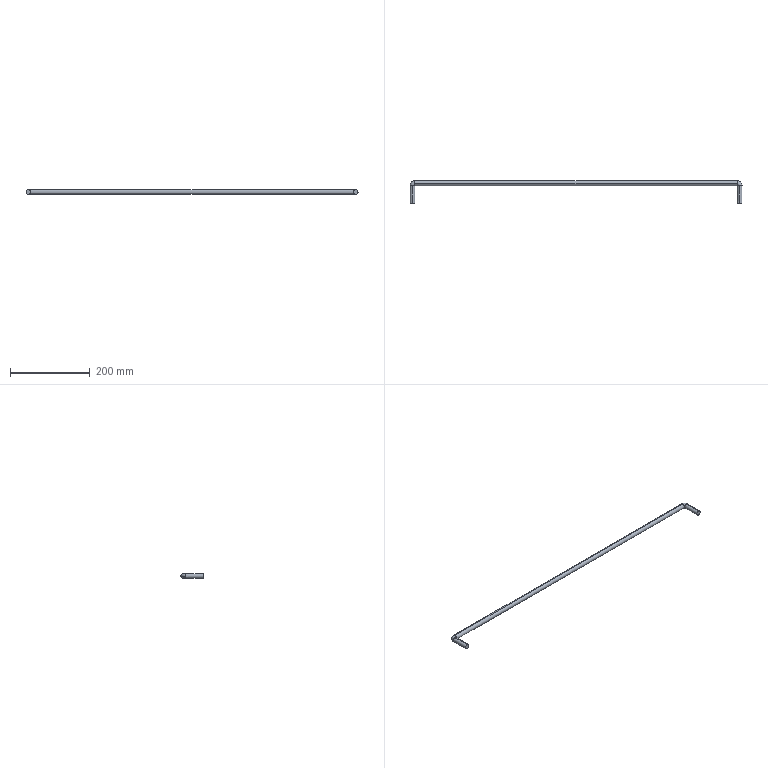Part | SolidWorks | features Sweep 1 | 1 solid | 12 faces | box 831 x 56 x 12 mm | volume 103305 mm3 | cylinder 6 | torus 4 | plane 2 | commonest cylinder face diameters 12 x6
STEP:
#1=CARTESIAN_POINT('',(-49.238,26.641,-6.));
#2=VERTEX_POINT('',#1);
#3=CARTESIAN_POINT('',(-55.238,26.641,0.));
#4=VERTEX_POINT('',#3);
#5=CARTESIAN_POINT('',(-49.238,26.641,0.));
#6=DIRECTION('',(0.,1.,0.));
#7=DIRECTION('',(0.,0.,1.));
#8=AXIS2_PLACEMENT_3D('',#5,#6,#7);
#9=CIRCLE('',#8,6.);
#10=EDGE_CURVE('',#2,#4,#9,.T.);
#11=ORIENTED_EDGE('',*,*,#10,.T.);
#12=CARTESIAN_POINT('',(-42.738,39.141,0.));
#13=VERTEX_POINT('',#12);
#14=CARTESIAN_POINT('',(-42.738,26.641,0.));
#15=DIRECTION('',(0.,0.,-1.));
#16=DIRECTION('',(-1.,0.,0.));
#17=AXIS2_PLACEMENT_3D('',#14,#15,#16);
#18=CIRCLE('',#17,12.5);
#19=EDGE_CURVE('',#4,#13,#18,.T.);
#20=ORIENTED_EDGE('',*,*,#19,.T.);
#21=CARTESIAN_POINT('',(-42.738,33.141,-6.));
#22=VERTEX_POINT('',#21);
#23=CARTESIAN_POINT('',(-42.738,33.141,0.));
#24=DIRECTION('',(1.,0.,0.));
#25=DIRECTION('',(0.,0.,1.));
#26=AXIS2_PLACEMENT_3D('',#23,#24,#25);
#27=CIRCLE('',#26,6.);
#28=EDGE_CURVE('',#22,#13,#27,.T.);
#29=ORIENTED_EDGE('',*,*,#28,.F.);
#30=CARTESIAN_POINT('',(-42.738,27.141,0.));
#31=VERTEX_POINT('',#30);
#32=CARTESIAN_POINT('',(-42.738,33.141,0.));
#33=DIRECTION('',(1.,0.,0.));
#34=DIRECTION('',(0.,0.,1.));
#35=AXIS2_PLACEMENT_3D('',#32,#33,#34);
#36=CIRCLE('',#35,6.);
#37=EDGE_CURVE('',#31,#22,#36,.T.);
#38=ORIENTED_EDGE('',*,*,#37,.F.);
#39=CARTESIAN_POINT('',(-43.238,26.641,0.));
#40=VERTEX_POINT('',#39);
#41=CARTESIAN_POINT('',(-42.738,26.641,0.));
#42=DIRECTION('',(0.,0.,-1.));
#43=DIRECTION('',(-1.,0.,0.));
#44=AXIS2_PLACEMENT_3D('',#41,#42,#43);
#45=CIRCLE('',#44,0.5);
#46=EDGE_CURVE('',#40,#31,#45,.T.);
#47=ORIENTED_EDGE('',*,*,#46,.F.);
#48=CARTESIAN_POINT('',(-49.238,26.641,0.));
#49=DIRECTION('',(0.,1.,0.));
#50=DIRECTION('',(0.,0.,1.));
#51=AXIS2_PLACEMENT_3D('',#48,#49,#50);
#52=CIRCLE('',#51,6.);
#53=EDGE_CURVE('',#40,#2,#52,.T.);
#54=ORIENTED_EDGE('',*,*,#53,.T.);
#55=EDGE_LOOP('',(#11,#20,#29,#38,#47,#54));
#56=FACE_OUTER_BOUND('',#55,.T.);
#57=CARTESIAN_POINT('',(-42.738,26.641,0.));
#58=DIRECTION('',(0.,0.,-1.));
#59=DIRECTION('',(-1.,0.,0.));
#60=AXIS2_PLACEMENT_3D('',#57,#58,#59);
#61=TOROIDAL_SURFACE('',#60,6.5,6.);
#62=ADVANCED_FACE('',(#56),#61,.T.);
#63=CARTESIAN_POINT('',(763.262,33.141,-6.));
#64=VERTEX_POINT('',#63);
#65=CARTESIAN_POINT('',(763.262,39.141,0.));
#66=VERTEX_POINT('',#65);
#67=CARTESIAN_POINT('',(763.262,33.141,0.));
#68=DIRECTION('',(1.,0.,0.));
#69=DIRECTION('',(0.,0.,1.));
#70=AXIS2_PLACEMENT_3D('',#67,#68,#69);
#71=CIRCLE('',#70,6.);
#72=EDGE_CURVE('',#64,#66,#71,.T.);
#73=ORIENTED_EDGE('',*,*,#72,.T.);
#74=CARTESIAN_POINT('',(775.762,26.641,0.));
#75=VERTEX_POINT('',#74);
#76=CARTESIAN_POINT('',(763.262,26.641,0.));
#77=DIRECTION('',(0.,0.,-1.));
#78=DIRECTION('',(-1.,0.,0.));
#79=AXIS2_PLACEMENT_3D('',#76,#77,#78);
#80=CIRCLE('',#79,12.5);
#81=EDGE_CURVE('',#66,#75,#80,.T.);
#82=ORIENTED_EDGE('',*,*,#81,.T.);
#83=CARTESIAN_POINT('',(769.762,26.641,-6.));
#84=VERTEX_POINT('',#83);
#85=CARTESIAN_POINT('',(769.762,26.641,0.));
#86=DIRECTION('',(0.,-1.,0.));
#87=DIRECTION('',(0.,0.,1.));
#88=AXIS2_PLACEMENT_3D('',#85,#86,#87);
#89=CIRCLE('',#88,6.);
#90=EDGE_CURVE('',#84,#75,#89,.T.);
#91=ORIENTED_EDGE('',*,*,#90,.F.);
#92=CARTESIAN_POINT('',(763.762,26.641,0.));
#93=VERTEX_POINT('',#92);
#94=CARTESIAN_POINT('',(769.762,26.641,0.));
#95=DIRECTION('',(0.,-1.,0.));
#96=DIRECTION('',(0.,0.,1.));
#97=AXIS2_PLACEMENT_3D('',#94,#95,#96);
#98=CIRCLE('',#97,6.);
#99=EDGE_CURVE('',#93,#84,#98,.T.);
#100=ORIENTED_EDGE('',*,*,#99,.F.);
#101=CARTESIAN_POINT('',(763.262,27.141,0.));
#102=VERTEX_POINT('',#101);
#103=CARTESIAN_POINT('',(763.262,26.641,0.));
#104=DIRECTION('',(0.,0.,-1.));
#105=DIRECTION('',(-1.,0.,0.));
#106=AXIS2_PLACEMENT_3D('',#103,#104,#105);
#107=CIRCLE('',#106,0.5);
#108=EDGE_CURVE('',#102,#93,#107,.T.);
#109=ORIENTED_EDGE('',*,*,#108,.F.);
#110=CARTESIAN_POINT('',(763.262,33.141,0.));
#111=DIRECTION('',(1.,0.,0.));
#112=DIRECTION('',(0.,0.,1.));
#113=AXIS2_PLACEMENT_3D('',#110,#111,#112);
#114=CIRCLE('',#113,6.);
#115=EDGE_CURVE('',#102,#64,#114,.T.);
#116=ORIENTED_EDGE('',*,*,#115,.T.);
#117=EDGE_LOOP('',(#73,#82,#91,#100,#109,#116));
#118=FACE_OUTER_BOUND('',#117,.T.);
#119=CARTESIAN_POINT('',(763.262,26.641,0.));
#120=DIRECTION('',(0.,0.,-1.));
#121=DIRECTION('',(-1.,0.,0.));
#122=AXIS2_PLACEMENT_3D('',#119,#120,#121);
#123=TOROIDAL_SURFACE('',#122,6.5,6.);
#124=ADVANCED_FACE('',(#118),#123,.T.);
#125=CARTESIAN_POINT('',(-49.238,26.641,6.));
#126=VERTEX_POINT('',#125);
#127=CARTESIAN_POINT('',(-49.238,26.641,0.));
#128=DIRECTION('',(0.,1.,0.));
#129=DIRECTION('',(0.,0.,1.));
#130=AXIS2_PLACEMENT_3D('',#127,#128,#129);
#131=CIRCLE('',#130,6.);
#132=EDGE_CURVE('',#126,#40,#131,.T.);
#133=ORIENTED_EDGE('',*,*,#132,.F.);
#134=CARTESIAN_POINT('',(-49.238,-16.859,6.));
#135=VERTEX_POINT('',#134);
#136=CARTESIAN_POINT('',(-49.238,26.641,6.));
#137=DIRECTION('',(0.,-1.,0.));
#138=VECTOR('',#137,1000.);
#139=LINE('',#136,#138);
#140=EDGE_CURVE('',#126,#135,#139,.T.);
#141=ORIENTED_EDGE('',*,*,#140,.T.);
#142=CARTESIAN_POINT('',(-49.238,-16.859,-6.));
#143=VERTEX_POINT('',#142);
#144=CARTESIAN_POINT('',(-49.238,-16.859,0.));
#145=DIRECTION('',(0.,1.,0.));
#146=DIRECTION('',(0.,0.,1.));
#147=AXIS2_PLACEMENT_3D('',#144,#145,#146);
#148=CIRCLE('',#147,6.);
#149=EDGE_CURVE('',#135,#143,#148,.T.);
#150=ORIENTED_EDGE('',*,*,#149,.T.);
#151=CARTESIAN_POINT('',(-49.238,26.641,-6.));
#152=DIRECTION('',(0.,-1.,0.));
#153=VECTOR('',#152,1000.);
#154=LINE('',#151,#153);
#155=EDGE_CURVE('',#2,#143,#154,.T.);
#156=ORIENTED_EDGE('',*,*,#155,.F.);
#157=ORIENTED_EDGE('',*,*,#53,.F.);
#158=EDGE_LOOP('',(#133,#141,#150,#156,#157));
#159=FACE_OUTER_BOUND('',#158,.T.);
#160=CARTESIAN_POINT('',(-49.238,26.641,0.));
#161=DIRECTION('',(0.,-1.,0.));
#162=DIRECTION('',(0.,0.,-1.));
#163=AXIS2_PLACEMENT_3D('',#160,#161,#162);
#164=CYLINDRICAL_SURFACE('',#163,6.);
#165=ADVANCED_FACE('',(#159),#164,.T.);
#166=ORIENTED_EDGE('',*,*,#28,.T.);
#167=CARTESIAN_POINT('',(-42.738,33.141,6.));
#168=VERTEX_POINT('',#167);
#169=CARTESIAN_POINT('',(-42.738,33.141,0.));
#170=DIRECTION('',(1.,0.,0.));
#171=DIRECTION('',(0.,0.,1.));
#172=AXIS2_PLACEMENT_3D('',#169,#170,#171);
#173=CIRCLE('',#172,6.);
#174=EDGE_CURVE('',#13,#168,#173,.T.);
#175=ORIENTED_EDGE('',*,*,#174,.T.);
#176=CARTESIAN_POINT('',(763.262,33.141,6.));
#177=VERTEX_POINT('',#176);
#178=CARTESIAN_POINT('',(-42.738,33.141,6.));
#179=DIRECTION('',(1.,0.,0.));
#180=VECTOR('',#179,1000.);
#181=LINE('',#178,#180);
#182=EDGE_CURVE('',#168,#177,#181,.T.);
#183=ORIENTED_EDGE('',*,*,#182,.T.);
#184=CARTESIAN_POINT('',(763.262,33.141,0.));
#185=DIRECTION('',(1.,0.,0.));
#186=DIRECTION('',(0.,0.,1.));
#187=AXIS2_PLACEMENT_3D('',#184,#185,#186);
#188=CIRCLE('',#187,6.);
#189=EDGE_CURVE('',#66,#177,#188,.T.);
#190=ORIENTED_EDGE('',*,*,#189,.F.);
#191=ORIENTED_EDGE('',*,*,#72,.F.);
#192=CARTESIAN_POINT('',(-42.738,33.141,-6.));
#193=DIRECTION('',(1.,0.,0.));
#194=VECTOR('',#193,1000.);
#195=LINE('',#192,#194);
#196=EDGE_CURVE('',#22,#64,#195,.T.);
#197=ORIENTED_EDGE('',*,*,#196,.F.);
#198=EDGE_LOOP('',(#166,#175,#183,#190,#191,#197));
#199=FACE_OUTER_BOUND('',#198,.T.);
#200=CARTESIAN_POINT('',(-42.738,33.141,0.));
#201=DIRECTION('',(1.,0.,0.));
#202=DIRECTION('',(0.,0.,-1.));
#203=AXIS2_PLACEMENT_3D('',#200,#201,#202);
#204=CYLINDRICAL_SURFACE('',#203,6.);
#205=ADVANCED_FACE('',(#199),#204,.T.);
#206=ORIENTED_EDGE('',*,*,#90,.T.);
#207=CARTESIAN_POINT('',(769.762,26.641,6.));
#208=VERTEX_POINT('',#207);
#209=CARTESIAN_POINT('',(769.762,26.641,0.));
#210=DIRECTION('',(0.,-1.,0.));
#211=DIRECTION('',(0.,0.,1.));
#212=AXIS2_PLACEMENT_3D('',#209,#210,#211);
#213=CIRCLE('',#212,6.);
#214=EDGE_CURVE('',#75,#208,#213,.T.);
#215=ORIENTED_EDGE('',*,*,#214,.T.);
#216=CARTESIAN_POINT('',(769.762,-16.859,6.));
#217=VERTEX_POINT('',#216);
#218=CARTESIAN_POINT('',(769.762,26.641,6.));
#219=DIRECTION('',(0.,-1.,0.));
#220=VECTOR('',#219,1000.);
#221=LINE('',#218,#220);
#222=EDGE_CURVE('',#208,#217,#221,.T.);
#223=ORIENTED_EDGE('',*,*,#222,.T.);
#224=CARTESIAN_POINT('',(769.762,-16.859,-6.));
#225=VERTEX_POINT('',#224);
#226=CARTESIAN_POINT('',(769.762,-16.859,0.));
#227=DIRECTION('',(0.,-1.,0.));
#228=DIRECTION('',(0.,0.,1.));
#229=AXIS2_PLACEMENT_3D('',#226,#227,#228);
#230=CIRCLE('',#229,6.);
#231=EDGE_CURVE('',#225,#217,#230,.T.);
#232=ORIENTED_EDGE('',*,*,#231,.F.);
#233=CARTESIAN_POINT('',(769.762,26.641,-6.));
#234=DIRECTION('',(0.,-1.,0.));
#235=VECTOR('',#234,1000.);
#236=LINE('',#233,#235);
#237=EDGE_CURVE('',#84,#225,#236,.T.);
#238=ORIENTED_EDGE('',*,*,#237,.F.);
#239=EDGE_LOOP('',(#206,#215,#223,#232,#238));
#240=FACE_OUTER_BOUND('',#239,.T.);
#241=CARTESIAN_POINT('',(769.762,26.641,0.));
#242=DIRECTION('',(0.,-1.,0.));
#243=DIRECTION('',(0.,0.,-1.));
#244=AXIS2_PLACEMENT_3D('',#241,#242,#243);
#245=CYLINDRICAL_SURFACE('',#244,6.);
#246=ADVANCED_FACE('',(#240),#245,.T.);
#247=ORIENTED_EDGE('',*,*,#222,.F.);
#248=CARTESIAN_POINT('',(769.762,26.641,0.));
#249=DIRECTION('',(0.,-1.,0.));
#250=DIRECTION('',(0.,0.,1.));
#251=AXIS2_PLACEMENT_3D('',#248,#249,#250);
#252=CIRCLE('',#251,6.);
#253=EDGE_CURVE('',#208,#93,#252,.T.);
#254=ORIENTED_EDGE('',*,*,#253,.T.);
#255=ORIENTED_EDGE('',*,*,#99,.T.);
#256=ORIENTED_EDGE('',*,*,#237,.T.);
#257=CARTESIAN_POINT('',(769.762,-16.859,0.));
#258=DIRECTION('',(0.,-1.,0.));
#259=DIRECTION('',(0.,0.,1.));
#260=AXIS2_PLACEMENT_3D('',#257,#258,#259);
#261=CIRCLE('',#260,6.);
#262=EDGE_CURVE('',#217,#225,#261,.T.);
#263=ORIENTED_EDGE('',*,*,#262,.F.);
#264=EDGE_LOOP('',(#247,#254,#255,#256,#263));
#265=FACE_OUTER_BOUND('',#264,.T.);
#266=CARTESIAN_POINT('',(769.762,26.641,0.));
#267=DIRECTION('',(0.,-1.,0.));
#268=DIRECTION('',(0.,0.,-1.));
#269=AXIS2_PLACEMENT_3D('',#266,#267,#268);
#270=CYLINDRICAL_SURFACE('',#269,6.);
#271=ADVANCED_FACE('',(#265),#270,.T.);
#272=ORIENTED_EDGE('',*,*,#81,.F.);
#273=ORIENTED_EDGE('',*,*,#189,.T.);
#274=CARTESIAN_POINT('',(763.262,33.141,0.));
#275=DIRECTION('',(1.,0.,0.));
#276=DIRECTION('',(0.,0.,1.));
#277=AXIS2_PLACEMENT_3D('',#274,#275,#276);
#278=CIRCLE('',#277,6.);
#279=EDGE_CURVE('',#177,#102,#278,.T.);
#280=ORIENTED_EDGE('',*,*,#279,.T.);
#281=ORIENTED_EDGE('',*,*,#108,.T.);
#282=ORIENTED_EDGE('',*,*,#253,.F.);
#283=ORIENTED_EDGE('',*,*,#214,.F.);
#284=EDGE_LOOP('',(#272,#273,#280,#281,#282,#283));
#285=FACE_OUTER_BOUND('',#284,.T.);
#286=CARTESIAN_POINT('',(763.262,26.641,0.));
#287=DIRECTION('',(0.,0.,-1.));
#288=DIRECTION('',(-1.,0.,0.));
#289=AXIS2_PLACEMENT_3D('',#286,#287,#288);
#290=TOROIDAL_SURFACE('',#289,6.5,6.);
#291=ADVANCED_FACE('',(#285),#290,.T.);
#292=ORIENTED_EDGE('',*,*,#182,.F.);
#293=CARTESIAN_POINT('',(-42.738,33.141,0.));
#294=DIRECTION('',(1.,0.,0.));
#295=DIRECTION('',(0.,0.,1.));
#296=AXIS2_PLACEMENT_3D('',#293,#294,#295);
#297=CIRCLE('',#296,6.);
#298=EDGE_CURVE('',#168,#31,#297,.T.);
#299=ORIENTED_EDGE('',*,*,#298,.T.);
#300=ORIENTED_EDGE('',*,*,#37,.T.);
#301=ORIENTED_EDGE('',*,*,#196,.T.);
#302=ORIENTED_EDGE('',*,*,#115,.F.);
#303=ORIENTED_EDGE('',*,*,#279,.F.);
#304=EDGE_LOOP('',(#292,#299,#300,#301,#302,#303));
#305=FACE_OUTER_BOUND('',#304,.T.);
#306=CARTESIAN_POINT('',(-42.738,33.141,0.));
#307=DIRECTION('',(1.,0.,0.));
#308=DIRECTION('',(0.,0.,-1.));
#309=AXIS2_PLACEMENT_3D('',#306,#307,#308);
#310=CYLINDRICAL_SURFACE('',#309,6.);
#311=ADVANCED_FACE('',(#305),#310,.T.);
#312=ORIENTED_EDGE('',*,*,#19,.F.);
#313=CARTESIAN_POINT('',(-49.238,26.641,0.));
#314=DIRECTION('',(0.,1.,0.));
#315=DIRECTION('',(0.,0.,1.));
#316=AXIS2_PLACEMENT_3D('',#313,#314,#315);
#317=CIRCLE('',#316,6.);
#318=EDGE_CURVE('',#4,#126,#317,.T.);
#319=ORIENTED_EDGE('',*,*,#318,.T.);
#320=ORIENTED_EDGE('',*,*,#132,.T.);
#321=ORIENTED_EDGE('',*,*,#46,.T.);
#322=ORIENTED_EDGE('',*,*,#298,.F.);
#323=ORIENTED_EDGE('',*,*,#174,.F.);
#324=EDGE_LOOP('',(#312,#319,#320,#321,#322,#323));
#325=FACE_OUTER_BOUND('',#324,.T.);
#326=CARTESIAN_POINT('',(-42.738,26.641,0.));
#327=DIRECTION('',(0.,0.,-1.));
#328=DIRECTION('',(-1.,0.,0.));
#329=AXIS2_PLACEMENT_3D('',#326,#327,#328);
#330=TOROIDAL_SURFACE('',#329,6.5,6.);
#331=ADVANCED_FACE('',(#325),#330,.T.);
#332=ORIENTED_EDGE('',*,*,#140,.F.);
#333=ORIENTED_EDGE('',*,*,#318,.F.);
#334=ORIENTED_EDGE('',*,*,#10,.F.);
#335=ORIENTED_EDGE('',*,*,#155,.T.);
#336=CARTESIAN_POINT('',(-49.238,-16.859,0.));
#337=DIRECTION('',(0.,1.,0.));
#338=DIRECTION('',(0.,0.,1.));
#339=AXIS2_PLACEMENT_3D('',#336,#337,#338);
#340=CIRCLE('',#339,6.);
#341=EDGE_CURVE('',#143,#135,#340,.T.);
#342=ORIENTED_EDGE('',*,*,#341,.T.);
#343=EDGE_LOOP('',(#332,#333,#334,#335,#342));
#344=FACE_OUTER_BOUND('',#343,.T.);
#345=CARTESIAN_POINT('',(-49.238,26.641,0.));
#346=DIRECTION('',(0.,-1.,0.));
#347=DIRECTION('',(0.,0.,-1.));
#348=AXIS2_PLACEMENT_3D('',#345,#346,#347);
#349=CYLINDRICAL_SURFACE('',#348,6.);
#350=ADVANCED_FACE('',(#344),#349,.T.);
#351=ORIENTED_EDGE('',*,*,#231,.T.);
#352=ORIENTED_EDGE('',*,*,#262,.T.);
#353=EDGE_LOOP('',(#351,#352));
#354=FACE_OUTER_BOUND('',#353,.T.);
#355=CARTESIAN_POINT('',(769.762,-16.859,0.));
#356=DIRECTION('',(0.,-1.,0.));
#357=DIRECTION('',(0.,0.,1.));
#358=AXIS2_PLACEMENT_3D('',#355,#356,#357);
#359=PLANE('',#358);
#360=ADVANCED_FACE('',(#354),#359,.T.);
#361=ORIENTED_EDGE('',*,*,#341,.F.);
#362=ORIENTED_EDGE('',*,*,#149,.F.);
#363=EDGE_LOOP('',(#361,#362));
#364=FACE_OUTER_BOUND('',#363,.T.);
#365=CARTESIAN_POINT('',(-49.238,-16.859,0.));
#366=DIRECTION('',(0.,1.,0.));
#367=DIRECTION('',(0.,0.,1.));
#368=AXIS2_PLACEMENT_3D('',#365,#366,#367);
#369=PLANE('',#368);
#370=ADVANCED_FACE('',(#364),#369,.F.);
#371=CLOSED_SHELL('',(#62,#124,#165,#205,#246,#271,#291,#311,#331,#350,#360,#370));
#372=MANIFOLD_SOLID_BREP('',#371);
#373=CARTESIAN_POINT('',(0.,0.,0.));
#374=DIRECTION('',(0.,0.,1.));
#375=DIRECTION('',(1.,0.,0.));
#376=AXIS2_PLACEMENT_3D('',#373,#374,#375);
#377=(LENGTH_UNIT()NAMED_UNIT(*)SI_UNIT(.MILLI.,.METRE.));
#378=UNCERTAINTY_MEASURE_WITH_UNIT(LENGTH_MEASURE(0.00001),#377,'','');
#379=(NAMED_UNIT(*)PLANE_ANGLE_UNIT()SI_UNIT($,.RADIAN.));
#380=(NAMED_UNIT(*)SI_UNIT($,.STERADIAN.)SOLID_ANGLE_UNIT());
#381=(GEOMETRIC_REPRESENTATION_CONTEXT(3)GLOBAL_UNCERTAINTY_ASSIGNED_CONTEXT((#378))GLOBAL_UNIT_ASSIGNED_CONTEXT((#377,#379,#380))REPRESENTATION_CONTEXT('',''));
#382=ADVANCED_BREP_SHAPE_REPRESENTATION('',(#372,#376),#381);